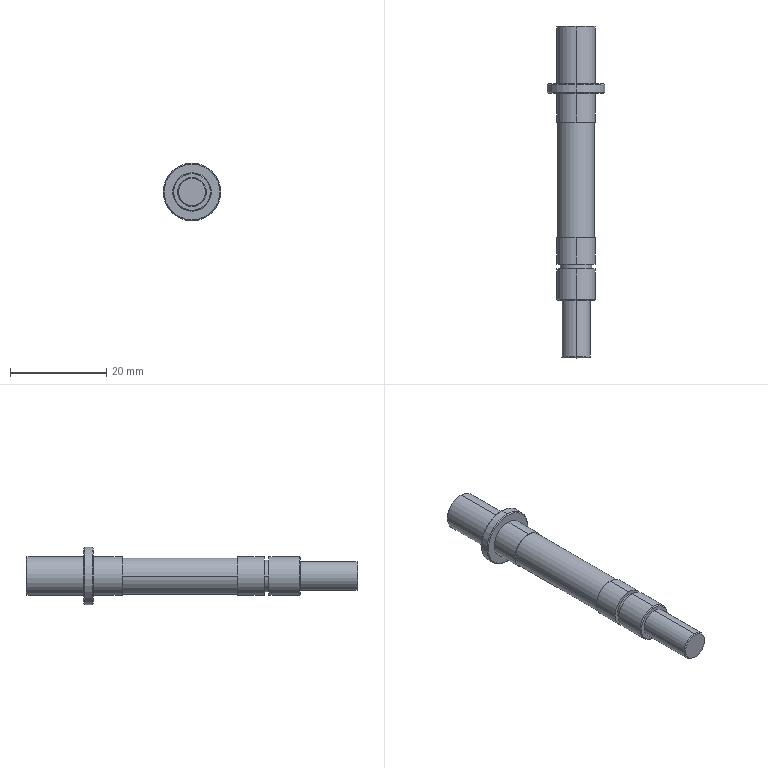Part | SolidWorks | features ICE 3, Chamfer 1, Extrusion 1, RevCut 1 | 1 solid | 35 faces | box 12 x 69 x 12 mm | volume 3193 mm3 | cylinder 16 | cone 10 | plane 9 | commonest cylinder face diameters 8 x8 6 x2 6.5 x2 7.6 x2 12 x2
STEP:
#1=CARTESIAN_POINT('',(0.,43.,-5.8));
#2=VERTEX_POINT('',#1);
#3=CARTESIAN_POINT('',(0.,43.,5.8));
#4=VERTEX_POINT('',#3);
#5=CARTESIAN_POINT('',(0.,43.,0.));
#6=DIRECTION('',(0.,-1.,0.));
#7=DIRECTION('',(0.,0.,1.));
#8=AXIS2_PLACEMENT_3D('',#5,#6,#7);
#9=CIRCLE('',#8,5.8);
#10=EDGE_CURVE('',#2,#4,#9,.T.);
#11=ORIENTED_EDGE('',*,*,#10,.F.);
#12=CARTESIAN_POINT('',(0.,43.2,-6.));
#13=VERTEX_POINT('',#12);
#14=CARTESIAN_POINT('',(0.,43.2,-6.));
#15=DIRECTION('',(0.,0.7071,-0.7071));
#16=VECTOR('',#15,1000.);
#17=LINE('',#14,#16);
#18=EDGE_CURVE('',#2,#13,#17,.T.);
#19=ORIENTED_EDGE('',*,*,#18,.T.);
#20=CARTESIAN_POINT('',(0.,43.2,6.));
#21=VERTEX_POINT('',#20);
#22=CARTESIAN_POINT('',(0.,43.2,0.));
#23=DIRECTION('',(0.,1.,0.));
#24=DIRECTION('',(0.,0.,1.));
#25=AXIS2_PLACEMENT_3D('',#22,#23,#24);
#26=CIRCLE('',#25,6.);
#27=EDGE_CURVE('',#21,#13,#26,.T.);
#28=ORIENTED_EDGE('',*,*,#27,.F.);
#29=CARTESIAN_POINT('',(0.,43.2,6.));
#30=DIRECTION('',(0.,0.7071,0.7071));
#31=VECTOR('',#30,1000.);
#32=LINE('',#29,#31);
#33=EDGE_CURVE('',#4,#21,#32,.T.);
#34=ORIENTED_EDGE('',*,*,#33,.F.);
#35=EDGE_LOOP('',(#11,#19,#28,#34));
#36=FACE_OUTER_BOUND('',#35,.T.);
#37=CARTESIAN_POINT('',(0.,43.2,0.));
#38=DIRECTION('',(0.,1.,0.));
#39=DIRECTION('',(0.,0.,1.));
#40=AXIS2_PLACEMENT_3D('',#37,#38,#39);
#41=CONICAL_SURFACE('',#40,6.,0.7854);
#42=ADVANCED_FACE('',(#36),#41,.T.);
#43=CARTESIAN_POINT('',(0.,0.,-3.8));
#44=VERTEX_POINT('',#43);
#45=CARTESIAN_POINT('',(0.,0.,3.8));
#46=VERTEX_POINT('',#45);
#47=CARTESIAN_POINT('',(0.,0.,0.));
#48=DIRECTION('',(0.,-1.,0.));
#49=DIRECTION('',(0.,0.,1.));
#50=AXIS2_PLACEMENT_3D('',#47,#48,#49);
#51=CIRCLE('',#50,3.8);
#52=EDGE_CURVE('',#44,#46,#51,.T.);
#53=ORIENTED_EDGE('',*,*,#52,.F.);
#54=CARTESIAN_POINT('',(0.,0.2,-4.));
#55=VERTEX_POINT('',#54);
#56=CARTESIAN_POINT('',(0.,0.2,-4.));
#57=DIRECTION('',(0.,0.7071,-0.7071));
#58=VECTOR('',#57,1000.);
#59=LINE('',#56,#58);
#60=EDGE_CURVE('',#44,#55,#59,.T.);
#61=ORIENTED_EDGE('',*,*,#60,.T.);
#62=CARTESIAN_POINT('',(0.,0.2,4.));
#63=VERTEX_POINT('',#62);
#64=CARTESIAN_POINT('',(0.,0.2,0.));
#65=DIRECTION('',(0.,1.,0.));
#66=DIRECTION('',(0.,0.,1.));
#67=AXIS2_PLACEMENT_3D('',#64,#65,#66);
#68=CIRCLE('',#67,4.);
#69=EDGE_CURVE('',#63,#55,#68,.T.);
#70=ORIENTED_EDGE('',*,*,#69,.F.);
#71=CARTESIAN_POINT('',(0.,0.2,4.));
#72=DIRECTION('',(0.,0.7071,0.7071));
#73=VECTOR('',#72,1000.);
#74=LINE('',#71,#73);
#75=EDGE_CURVE('',#46,#63,#74,.T.);
#76=ORIENTED_EDGE('',*,*,#75,.F.);
#77=EDGE_LOOP('',(#53,#61,#70,#76));
#78=FACE_OUTER_BOUND('',#77,.T.);
#79=CARTESIAN_POINT('',(0.,0.2,0.));
#80=DIRECTION('',(0.,1.,0.));
#81=DIRECTION('',(0.,0.,1.));
#82=AXIS2_PLACEMENT_3D('',#79,#80,#81);
#83=CONICAL_SURFACE('',#82,4.,0.7854);
#84=ADVANCED_FACE('',(#78),#83,.T.);
#85=CARTESIAN_POINT('',(0.,-12.,-2.8));
#86=VERTEX_POINT('',#85);
#87=CARTESIAN_POINT('',(0.,-12.,2.8));
#88=VERTEX_POINT('',#87);
#89=CARTESIAN_POINT('',(0.,-12.,0.));
#90=DIRECTION('',(0.,-1.,0.));
#91=DIRECTION('',(0.,0.,-1.));
#92=AXIS2_PLACEMENT_3D('',#89,#90,#91);
#93=CIRCLE('',#92,2.8);
#94=EDGE_CURVE('',#86,#88,#93,.T.);
#95=ORIENTED_EDGE('',*,*,#94,.F.);
#96=CARTESIAN_POINT('',(0.,-11.8,-3.));
#97=VERTEX_POINT('',#96);
#98=CARTESIAN_POINT('',(0.,-12.,-2.8));
#99=DIRECTION('',(0.,0.7071,-0.7071));
#100=VECTOR('',#99,1000.);
#101=LINE('',#98,#100);
#102=EDGE_CURVE('',#86,#97,#101,.T.);
#103=ORIENTED_EDGE('',*,*,#102,.T.);
#104=CARTESIAN_POINT('',(0.,-11.8,3.));
#105=VERTEX_POINT('',#104);
#106=CARTESIAN_POINT('',(0.,-11.8,0.));
#107=DIRECTION('',(0.,1.,0.));
#108=DIRECTION('',(0.,0.,-1.));
#109=AXIS2_PLACEMENT_3D('',#106,#107,#108);
#110=CIRCLE('',#109,3.);
#111=EDGE_CURVE('',#105,#97,#110,.T.);
#112=ORIENTED_EDGE('',*,*,#111,.F.);
#113=CARTESIAN_POINT('',(0.,-12.,2.8));
#114=DIRECTION('',(0.,0.7071,0.7071));
#115=VECTOR('',#114,1000.);
#116=LINE('',#113,#115);
#117=EDGE_CURVE('',#88,#105,#116,.T.);
#118=ORIENTED_EDGE('',*,*,#117,.F.);
#119=EDGE_LOOP('',(#95,#103,#112,#118));
#120=FACE_OUTER_BOUND('',#119,.T.);
#121=CARTESIAN_POINT('',(0.,-12.,0.));
#122=DIRECTION('',(0.,1.,0.));
#123=DIRECTION('',(0.,0.,1.));
#124=AXIS2_PLACEMENT_3D('',#121,#122,#123);
#125=CONICAL_SURFACE('',#124,2.8,0.7854);
#126=ADVANCED_FACE('',(#120),#125,.T.);
#127=CARTESIAN_POINT('',(0.,57.,3.8));
#128=VERTEX_POINT('',#127);
#129=CARTESIAN_POINT('',(0.,57.,-3.8));
#130=VERTEX_POINT('',#129);
#131=CARTESIAN_POINT('',(0.,57.,0.));
#132=DIRECTION('',(0.,1.,0.));
#133=DIRECTION('',(0.,0.,1.));
#134=AXIS2_PLACEMENT_3D('',#131,#132,#133);
#135=CIRCLE('',#134,3.8);
#136=EDGE_CURVE('',#128,#130,#135,.T.);
#137=ORIENTED_EDGE('',*,*,#136,.F.);
#138=CARTESIAN_POINT('',(0.,56.8,4.));
#139=VERTEX_POINT('',#138);
#140=CARTESIAN_POINT('',(0.,57.,3.8));
#141=DIRECTION('',(0.,-0.7071,0.7071));
#142=VECTOR('',#141,1000.);
#143=LINE('',#140,#142);
#144=EDGE_CURVE('',#128,#139,#143,.T.);
#145=ORIENTED_EDGE('',*,*,#144,.T.);
#146=CARTESIAN_POINT('',(0.,56.8,-4.));
#147=VERTEX_POINT('',#146);
#148=CARTESIAN_POINT('',(0.,56.8,0.));
#149=DIRECTION('',(0.,-1.,0.));
#150=DIRECTION('',(0.,0.,1.));
#151=AXIS2_PLACEMENT_3D('',#148,#149,#150);
#152=CIRCLE('',#151,4.);
#153=EDGE_CURVE('',#147,#139,#152,.T.);
#154=ORIENTED_EDGE('',*,*,#153,.F.);
#155=CARTESIAN_POINT('',(0.,57.,-3.8));
#156=DIRECTION('',(0.,-0.7071,-0.7071));
#157=VECTOR('',#156,1000.);
#158=LINE('',#155,#157);
#159=EDGE_CURVE('',#130,#147,#158,.T.);
#160=ORIENTED_EDGE('',*,*,#159,.F.);
#161=EDGE_LOOP('',(#137,#145,#154,#160));
#162=FACE_OUTER_BOUND('',#161,.T.);
#163=CARTESIAN_POINT('',(0.,57.,0.));
#164=DIRECTION('',(0.,-1.,0.));
#165=DIRECTION('',(0.,0.,-1.));
#166=AXIS2_PLACEMENT_3D('',#163,#164,#165);
#167=CONICAL_SURFACE('',#166,3.8,0.7854);
#168=ADVANCED_FACE('',(#162),#167,.T.);
#169=CARTESIAN_POINT('',(0.,45.,5.8));
#170=VERTEX_POINT('',#169);
#171=CARTESIAN_POINT('',(0.,45.,-5.8));
#172=VERTEX_POINT('',#171);
#173=CARTESIAN_POINT('',(0.,45.,0.));
#174=DIRECTION('',(0.,1.,0.));
#175=DIRECTION('',(0.,0.,1.));
#176=AXIS2_PLACEMENT_3D('',#173,#174,#175);
#177=CIRCLE('',#176,5.8);
#178=EDGE_CURVE('',#170,#172,#177,.T.);
#179=ORIENTED_EDGE('',*,*,#178,.F.);
#180=CARTESIAN_POINT('',(0.,44.8,6.));
#181=VERTEX_POINT('',#180);
#182=CARTESIAN_POINT('',(0.,45.,5.8));
#183=DIRECTION('',(0.,-0.7071,0.7071));
#184=VECTOR('',#183,1000.);
#185=LINE('',#182,#184);
#186=EDGE_CURVE('',#170,#181,#185,.T.);
#187=ORIENTED_EDGE('',*,*,#186,.T.);
#188=CARTESIAN_POINT('',(0.,44.8,-6.));
#189=VERTEX_POINT('',#188);
#190=CARTESIAN_POINT('',(0.,44.8,0.));
#191=DIRECTION('',(0.,-1.,0.));
#192=DIRECTION('',(0.,0.,1.));
#193=AXIS2_PLACEMENT_3D('',#190,#191,#192);
#194=CIRCLE('',#193,6.);
#195=EDGE_CURVE('',#189,#181,#194,.T.);
#196=ORIENTED_EDGE('',*,*,#195,.F.);
#197=CARTESIAN_POINT('',(0.,45.,-5.8));
#198=DIRECTION('',(0.,-0.7071,-0.7071));
#199=VECTOR('',#198,1000.);
#200=LINE('',#197,#199);
#201=EDGE_CURVE('',#172,#189,#200,.T.);
#202=ORIENTED_EDGE('',*,*,#201,.F.);
#203=EDGE_LOOP('',(#179,#187,#196,#202));
#204=FACE_OUTER_BOUND('',#203,.T.);
#205=CARTESIAN_POINT('',(0.,45.,0.));
#206=DIRECTION('',(0.,-1.,0.));
#207=DIRECTION('',(0.,0.,-1.));
#208=AXIS2_PLACEMENT_3D('',#205,#206,#207);
#209=CONICAL_SURFACE('',#208,5.8,0.7854);
#210=ADVANCED_FACE('',(#204),#209,.T.);
#211=ORIENTED_EDGE('',*,*,#111,.T.);
#212=CARTESIAN_POINT('',(0.,0.,-3.));
#213=VERTEX_POINT('',#212);
#214=CARTESIAN_POINT('',(0.,-12.,-3.));
#215=DIRECTION('',(0.,1.,0.));
#216=VECTOR('',#215,1000.);
#217=LINE('',#214,#216);
#218=EDGE_CURVE('',#97,#213,#217,.T.);
#219=ORIENTED_EDGE('',*,*,#218,.T.);
#220=CARTESIAN_POINT('',(0.,0.,3.));
#221=VERTEX_POINT('',#220);
#222=CARTESIAN_POINT('',(0.,0.,0.));
#223=DIRECTION('',(0.,-1.,0.));
#224=DIRECTION('',(0.,0.,1.));
#225=AXIS2_PLACEMENT_3D('',#222,#223,#224);
#226=CIRCLE('',#225,3.);
#227=EDGE_CURVE('',#213,#221,#226,.T.);
#228=ORIENTED_EDGE('',*,*,#227,.T.);
#229=CARTESIAN_POINT('',(0.,-12.,3.));
#230=DIRECTION('',(0.,1.,0.));
#231=VECTOR('',#230,1000.);
#232=LINE('',#229,#231);
#233=EDGE_CURVE('',#105,#221,#232,.T.);
#234=ORIENTED_EDGE('',*,*,#233,.F.);
#235=EDGE_LOOP('',(#211,#219,#228,#234));
#236=FACE_OUTER_BOUND('',#235,.T.);
#237=CARTESIAN_POINT('',(0.,-12.,0.));
#238=DIRECTION('',(0.,1.,0.));
#239=DIRECTION('',(0.,0.,1.));
#240=AXIS2_PLACEMENT_3D('',#237,#238,#239);
#241=CYLINDRICAL_SURFACE('',#240,3.);
#242=ADVANCED_FACE('',(#236),#241,.T.);
#243=CARTESIAN_POINT('',(0.,6.5,-4.));
#244=VERTEX_POINT('',#243);
#245=CARTESIAN_POINT('',(0.,6.5,4.));
#246=VERTEX_POINT('',#245);
#247=CARTESIAN_POINT('',(0.,6.5,0.));
#248=DIRECTION('',(0.,-1.,0.));
#249=DIRECTION('',(1.,0.,0.));
#250=AXIS2_PLACEMENT_3D('',#247,#248,#249);
#251=CIRCLE('',#250,4.);
#252=EDGE_CURVE('',#244,#246,#251,.T.);
#253=ORIENTED_EDGE('',*,*,#252,.T.);
#254=CARTESIAN_POINT('',(0.,43.,4.));
#255=DIRECTION('',(0.,-1.,0.));
#256=VECTOR('',#255,1000.);
#257=LINE('',#254,#256);
#258=EDGE_CURVE('',#246,#63,#257,.T.);
#259=ORIENTED_EDGE('',*,*,#258,.T.);
#260=ORIENTED_EDGE('',*,*,#69,.T.);
#261=CARTESIAN_POINT('',(0.,43.,-4.));
#262=DIRECTION('',(0.,-1.,0.));
#263=VECTOR('',#262,1000.);
#264=LINE('',#261,#263);
#265=EDGE_CURVE('',#244,#55,#264,.T.);
#266=ORIENTED_EDGE('',*,*,#265,.F.);
#267=EDGE_LOOP('',(#253,#259,#260,#266));
#268=FACE_OUTER_BOUND('',#267,.T.);
#269=CARTESIAN_POINT('',(0.,43.,0.));
#270=DIRECTION('',(0.,-1.,0.));
#271=DIRECTION('',(0.,0.,-1.));
#272=AXIS2_PLACEMENT_3D('',#269,#270,#271);
#273=CYLINDRICAL_SURFACE('',#272,4.);
#274=ADVANCED_FACE('',(#268),#273,.T.);
#275=CARTESIAN_POINT('',(3.25,7.5,0.));
#276=VERTEX_POINT('',#275);
#277=CARTESIAN_POINT('',(-3.25,7.5,0.));
#278=VERTEX_POINT('',#277);
#279=CARTESIAN_POINT('',(0.,7.5,0.));
#280=DIRECTION('',(0.,-1.,0.));
#281=DIRECTION('',(1.,0.,0.));
#282=AXIS2_PLACEMENT_3D('',#279,#280,#281);
#283=CIRCLE('',#282,3.25);
#284=EDGE_CURVE('',#276,#278,#283,.T.);
#285=ORIENTED_EDGE('',*,*,#284,.T.);
#286=CARTESIAN_POINT('',(-3.25,6.5,0.));
#287=VERTEX_POINT('',#286);
#288=CARTESIAN_POINT('',(-3.25,0.,0.));
#289=DIRECTION('',(0.,-1.,0.));
#290=VECTOR('',#289,1000.);
#291=LINE('',#288,#290);
#292=EDGE_CURVE('',#278,#287,#291,.T.);
#293=ORIENTED_EDGE('',*,*,#292,.T.);
#294=CARTESIAN_POINT('',(3.25,6.5,0.));
#295=VERTEX_POINT('',#294);
#296=CARTESIAN_POINT('',(0.,6.5,0.));
#297=DIRECTION('',(0.,-1.,0.));
#298=DIRECTION('',(1.,0.,0.));
#299=AXIS2_PLACEMENT_3D('',#296,#297,#298);
#300=CIRCLE('',#299,3.25);
#301=EDGE_CURVE('',#295,#287,#300,.T.);
#302=ORIENTED_EDGE('',*,*,#301,.F.);
#303=CARTESIAN_POINT('',(3.25,0.,0.));
#304=DIRECTION('',(0.,-1.,0.));
#305=VECTOR('',#304,1000.);
#306=LINE('',#303,#305);
#307=EDGE_CURVE('',#276,#295,#306,.T.);
#308=ORIENTED_EDGE('',*,*,#307,.F.);
#309=EDGE_LOOP('',(#285,#293,#302,#308));
#310=FACE_OUTER_BOUND('',#309,.T.);
#311=CARTESIAN_POINT('',(0.,0.,0.));
#312=DIRECTION('',(0.,-1.,0.));
#313=DIRECTION('',(1.,0.,0.));
#314=AXIS2_PLACEMENT_3D('',#311,#312,#313);
#315=CYLINDRICAL_SURFACE('',#314,3.25);
#316=ADVANCED_FACE('',(#310),#315,.T.);
#317=CARTESIAN_POINT('',(0.,13.,-4.));
#318=VERTEX_POINT('',#317);
#319=CARTESIAN_POINT('',(0.,13.,4.));
#320=VERTEX_POINT('',#319);
#321=CARTESIAN_POINT('',(0.,13.,0.));
#322=DIRECTION('',(0.,-1.,0.));
#323=DIRECTION('',(1.,0.,0.));
#324=AXIS2_PLACEMENT_3D('',#321,#322,#323);
#325=CIRCLE('',#324,4.);
#326=EDGE_CURVE('',#318,#320,#325,.T.);
#327=ORIENTED_EDGE('',*,*,#326,.T.);
#328=CARTESIAN_POINT('',(0.,7.5,4.));
#329=VERTEX_POINT('',#328);
#330=CARTESIAN_POINT('',(0.,43.,4.));
#331=DIRECTION('',(0.,-1.,0.));
#332=VECTOR('',#331,1000.);
#333=LINE('',#330,#332);
#334=EDGE_CURVE('',#320,#329,#333,.T.);
#335=ORIENTED_EDGE('',*,*,#334,.T.);
#336=CARTESIAN_POINT('',(0.,7.5,-4.));
#337=VERTEX_POINT('',#336);
#338=CARTESIAN_POINT('',(0.,7.5,0.));
#339=DIRECTION('',(0.,1.,0.));
#340=DIRECTION('',(-1.,0.,0.));
#341=AXIS2_PLACEMENT_3D('',#338,#339,#340);
#342=CIRCLE('',#341,4.);
#343=EDGE_CURVE('',#329,#337,#342,.T.);
#344=ORIENTED_EDGE('',*,*,#343,.T.);
#345=CARTESIAN_POINT('',(0.,43.,-4.));
#346=DIRECTION('',(0.,-1.,0.));
#347=VECTOR('',#346,1000.);
#348=LINE('',#345,#347);
#349=EDGE_CURVE('',#318,#337,#348,.T.);
#350=ORIENTED_EDGE('',*,*,#349,.F.);
#351=EDGE_LOOP('',(#327,#335,#344,#350));
#352=FACE_OUTER_BOUND('',#351,.T.);
#353=CARTESIAN_POINT('',(0.,43.,0.));
#354=DIRECTION('',(0.,-1.,0.));
#355=DIRECTION('',(0.,0.,-1.));
#356=AXIS2_PLACEMENT_3D('',#353,#354,#355);
#357=CYLINDRICAL_SURFACE('',#356,4.);
#358=ADVANCED_FACE('',(#352),#357,.T.);
#359=CARTESIAN_POINT('',(3.8,37.,0.));
#360=VERTEX_POINT('',#359);
#361=CARTESIAN_POINT('',(-3.8,37.,0.));
#362=VERTEX_POINT('',#361);
#363=CARTESIAN_POINT('',(0.,37.,0.));
#364=DIRECTION('',(0.,-1.,0.));
#365=DIRECTION('',(1.,0.,0.));
#366=AXIS2_PLACEMENT_3D('',#363,#364,#365);
#367=CIRCLE('',#366,3.8);
#368=EDGE_CURVE('',#360,#362,#367,.T.);
#369=ORIENTED_EDGE('',*,*,#368,.T.);
#370=CARTESIAN_POINT('',(-3.8,13.,0.));
#371=VERTEX_POINT('',#370);
#372=CARTESIAN_POINT('',(-3.8,0.,0.));
#373=DIRECTION('',(0.,-1.,0.));
#374=VECTOR('',#373,1000.);
#375=LINE('',#372,#374);
#376=EDGE_CURVE('',#362,#371,#375,.T.);
#377=ORIENTED_EDGE('',*,*,#376,.T.);
#378=CARTESIAN_POINT('',(3.8,13.,0.));
#379=VERTEX_POINT('',#378);
#380=CARTESIAN_POINT('',(0.,13.,0.));
#381=DIRECTION('',(0.,-1.,0.));
#382=DIRECTION('',(1.,0.,0.));
#383=AXIS2_PLACEMENT_3D('',#380,#381,#382);
#384=CIRCLE('',#383,3.8);
#385=EDGE_CURVE('',#379,#371,#384,.T.);
#386=ORIENTED_EDGE('',*,*,#385,.F.);
#387=CARTESIAN_POINT('',(3.8,0.,0.));
#388=DIRECTION('',(0.,-1.,0.));
#389=VECTOR('',#388,1000.);
#390=LINE('',#387,#389);
#391=EDGE_CURVE('',#360,#379,#390,.T.);
#392=ORIENTED_EDGE('',*,*,#391,.F.);
#393=EDGE_LOOP('',(#369,#377,#386,#392));
#394=FACE_OUTER_BOUND('',#393,.T.);
#395=CARTESIAN_POINT('',(0.,0.,0.));
#396=DIRECTION('',(0.,-1.,0.));
#397=DIRECTION('',(1.,0.,0.));
#398=AXIS2_PLACEMENT_3D('',#395,#396,#397);
#399=CYLINDRICAL_SURFACE('',#398,3.8);
#400=ADVANCED_FACE('',(#394),#399,.T.);
#401=ORIENTED_EDGE('',*,*,#153,.T.);
#402=CARTESIAN_POINT('',(0.,45.,4.));
#403=VERTEX_POINT('',#402);
#404=CARTESIAN_POINT('',(0.,57.,4.));
#405=DIRECTION('',(0.,-1.,0.));
#406=VECTOR('',#405,1000.);
#407=LINE('',#404,#406);
#408=EDGE_CURVE('',#139,#403,#407,.T.);
#409=ORIENTED_EDGE('',*,*,#408,.T.);
#410=CARTESIAN_POINT('',(0.,45.,-4.));
#411=VERTEX_POINT('',#410);
#412=CARTESIAN_POINT('',(0.,45.,0.));
#413=DIRECTION('',(0.,1.,0.));
#414=DIRECTION('',(0.,0.,1.));
#415=AXIS2_PLACEMENT_3D('',#412,#413,#414);
#416=CIRCLE('',#415,4.);
#417=EDGE_CURVE('',#403,#411,#416,.T.);
#418=ORIENTED_EDGE('',*,*,#417,.T.);
#419=CARTESIAN_POINT('',(0.,57.,-4.));
#420=DIRECTION('',(0.,-1.,0.));
#421=VECTOR('',#420,1000.);
#422=LINE('',#419,#421);
#423=EDGE_CURVE('',#147,#411,#422,.T.);
#424=ORIENTED_EDGE('',*,*,#423,.F.);
#425=EDGE_LOOP('',(#401,#409,#418,#424));
#426=FACE_OUTER_BOUND('',#425,.T.);
#427=CARTESIAN_POINT('',(0.,57.,0.));
#428=DIRECTION('',(0.,-1.,0.));
#429=DIRECTION('',(0.,0.,-1.));
#430=AXIS2_PLACEMENT_3D('',#427,#428,#429);
#431=CYLINDRICAL_SURFACE('',#430,4.);
#432=ADVANCED_FACE('',(#426),#431,.T.);
#433=ORIENTED_EDGE('',*,*,#195,.T.);
#434=CARTESIAN_POINT('',(0.,45.,6.));
#435=DIRECTION('',(0.,-1.,0.));
#436=VECTOR('',#435,1000.);
#437=LINE('',#434,#436);
#438=EDGE_CURVE('',#181,#21,#437,.T.);
#439=ORIENTED_EDGE('',*,*,#438,.T.);
#440=ORIENTED_EDGE('',*,*,#27,.T.);
#441=CARTESIAN_POINT('',(0.,45.,-6.));
#442=DIRECTION('',(0.,-1.,0.));
#443=VECTOR('',#442,1000.);
#444=LINE('',#441,#443);
#445=EDGE_CURVE('',#189,#13,#444,.T.);
#446=ORIENTED_EDGE('',*,*,#445,.F.);
#447=EDGE_LOOP('',(#433,#439,#440,#446));
#448=FACE_OUTER_BOUND('',#447,.T.);
#449=CARTESIAN_POINT('',(0.,45.,0.));
#450=DIRECTION('',(0.,-1.,0.));
#451=DIRECTION('',(0.,0.,-1.));
#452=AXIS2_PLACEMENT_3D('',#449,#450,#451);
#453=CYLINDRICAL_SURFACE('',#452,6.);
#454=ADVANCED_FACE('',(#448),#453,.T.);
#455=CARTESIAN_POINT('',(0.,43.,4.));
#456=VERTEX_POINT('',#455);
#457=CARTESIAN_POINT('',(0.,43.,-4.));
#458=VERTEX_POINT('',#457);
#459=CARTESIAN_POINT('',(0.,43.,0.));
#460=DIRECTION('',(0.,1.,0.));
#461=DIRECTION('',(0.,0.,1.));
#462=AXIS2_PLACEMENT_3D('',#459,#460,#461);
#463=CIRCLE('',#462,4.);
#464=EDGE_CURVE('',#456,#458,#463,.T.);
#465=ORIENTED_EDGE('',*,*,#464,.F.);
#466=CARTESIAN_POINT('',(0.,37.,4.));
#467=VERTEX_POINT('',#466);
#468=CARTESIAN_POINT('',(0.,43.,4.));
#469=DIRECTION('',(0.,-1.,0.));
#470=VECTOR('',#469,1000.);
#471=LINE('',#468,#470);
#472=EDGE_CURVE('',#456,#467,#471,.T.);
#473=ORIENTED_EDGE('',*,*,#472,.T.);
#474=CARTESIAN_POINT('',(0.,37.,-4.));
#475=VERTEX_POINT('',#474);
#476=CARTESIAN_POINT('',(0.,37.,0.));
#477=DIRECTION('',(0.,1.,0.));
#478=DIRECTION('',(-1.,0.,0.));
#479=AXIS2_PLACEMENT_3D('',#476,#477,#478);
#480=CIRCLE('',#479,4.);
#481=EDGE_CURVE('',#467,#475,#480,.T.);
#482=ORIENTED_EDGE('',*,*,#481,.T.);
#483=CARTESIAN_POINT('',(0.,43.,-4.));
#484=DIRECTION('',(0.,-1.,0.));
#485=VECTOR('',#484,1000.);
#486=LINE('',#483,#485);
#487=EDGE_CURVE('',#458,#475,#486,.T.);
#488=ORIENTED_EDGE('',*,*,#487,.F.);
#489=EDGE_LOOP('',(#465,#473,#482,#488));
#490=FACE_OUTER_BOUND('',#489,.T.);
#491=CARTESIAN_POINT('',(0.,43.,0.));
#492=DIRECTION('',(0.,-1.,0.));
#493=DIRECTION('',(0.,0.,-1.));
#494=AXIS2_PLACEMENT_3D('',#491,#492,#493);
#495=CYLINDRICAL_SURFACE('',#494,4.);
#496=ADVANCED_FACE('',(#490),#495,.T.);
#497=CARTESIAN_POINT('',(0.,0.,0.));
#498=DIRECTION('',(0.,-1.,0.));
#499=DIRECTION('',(0.,0.,1.));
#500=AXIS2_PLACEMENT_3D('',#497,#498,#499);
#501=CIRCLE('',#500,3.8);
#502=EDGE_CURVE('',#46,#44,#501,.T.);
#503=ORIENTED_EDGE('',*,*,#502,.T.);
#504=ORIENTED_EDGE('',*,*,#52,.T.);
#505=EDGE_LOOP('',(#503,#504));
#506=FACE_OUTER_BOUND('',#505,.T.);
#507=CARTESIAN_POINT('',(0.,0.,0.));
#508=DIRECTION('',(0.,-1.,0.));
#509=DIRECTION('',(0.,0.,1.));
#510=AXIS2_PLACEMENT_3D('',#507,#508,#509);
#511=CIRCLE('',#510,3.);
#512=EDGE_CURVE('',#221,#213,#511,.T.);
#513=ORIENTED_EDGE('',*,*,#512,.F.);
#514=ORIENTED_EDGE('',*,*,#227,.F.);
#515=EDGE_LOOP('',(#513,#514));
#516=FACE_BOUND('',#515,.T.);
#517=CARTESIAN_POINT('',(0.,0.,0.));
#518=DIRECTION('',(0.,1.,0.));
#519=DIRECTION('',(0.,0.,1.));
#520=AXIS2_PLACEMENT_3D('',#517,#518,#519);
#521=PLANE('',#520);
#522=ADVANCED_FACE('',(#506,#516),#521,.F.);
#523=CARTESIAN_POINT('',(0.,45.,0.));
#524=DIRECTION('',(0.,1.,0.));
#525=DIRECTION('',(0.,0.,1.));
#526=AXIS2_PLACEMENT_3D('',#523,#524,#525);
#527=CIRCLE('',#526,5.8);
#528=EDGE_CURVE('',#172,#170,#527,.T.);
#529=ORIENTED_EDGE('',*,*,#528,.T.);
#530=ORIENTED_EDGE('',*,*,#178,.T.);
#531=EDGE_LOOP('',(#529,#530));
#532=FACE_OUTER_BOUND('',#531,.T.);
#533=CARTESIAN_POINT('',(0.,45.,0.));
#534=DIRECTION('',(0.,1.,0.));
#535=DIRECTION('',(0.,0.,1.));
#536=AXIS2_PLACEMENT_3D('',#533,#534,#535);
#537=CIRCLE('',#536,4.);
#538=EDGE_CURVE('',#411,#403,#537,.T.);
#539=ORIENTED_EDGE('',*,*,#538,.F.);
#540=ORIENTED_EDGE('',*,*,#417,.F.);
#541=EDGE_LOOP('',(#539,#540));
#542=FACE_BOUND('',#541,.T.);
#543=CARTESIAN_POINT('',(0.,45.,0.));
#544=DIRECTION('',(0.,1.,0.));
#545=DIRECTION('',(0.,0.,1.));
#546=AXIS2_PLACEMENT_3D('',#543,#544,#545);
#547=PLANE('',#546);
#548=ADVANCED_FACE('',(#532,#542),#547,.T.);
#549=ORIENTED_EDGE('',*,*,#472,.F.);
#550=CARTESIAN_POINT('',(0.,43.,0.));
#551=DIRECTION('',(0.,1.,0.));
#552=DIRECTION('',(0.,0.,1.));
#553=AXIS2_PLACEMENT_3D('',#550,#551,#552);
#554=CIRCLE('',#553,4.);
#555=EDGE_CURVE('',#458,#456,#554,.T.);
#556=ORIENTED_EDGE('',*,*,#555,.F.);
#557=ORIENTED_EDGE('',*,*,#487,.T.);
#558=CARTESIAN_POINT('',(0.,37.,0.));
#559=DIRECTION('',(0.,1.,0.));
#560=DIRECTION('',(-1.,0.,0.));
#561=AXIS2_PLACEMENT_3D('',#558,#559,#560);
#562=CIRCLE('',#561,4.);
#563=EDGE_CURVE('',#475,#467,#562,.T.);
#564=ORIENTED_EDGE('',*,*,#563,.T.);
#565=EDGE_LOOP('',(#549,#556,#557,#564));
#566=FACE_OUTER_BOUND('',#565,.T.);
#567=CARTESIAN_POINT('',(0.,43.,0.));
#568=DIRECTION('',(0.,-1.,0.));
#569=DIRECTION('',(0.,0.,-1.));
#570=AXIS2_PLACEMENT_3D('',#567,#568,#569);
#571=CYLINDRICAL_SURFACE('',#570,4.);
#572=ADVANCED_FACE('',(#566),#571,.T.);
#573=CARTESIAN_POINT('',(0.,43.,0.));
#574=DIRECTION('',(0.,-1.,0.));
#575=DIRECTION('',(0.,0.,1.));
#576=AXIS2_PLACEMENT_3D('',#573,#574,#575);
#577=CIRCLE('',#576,5.8);
#578=EDGE_CURVE('',#4,#2,#577,.T.);
#579=ORIENTED_EDGE('',*,*,#578,.T.);
#580=ORIENTED_EDGE('',*,*,#10,.T.);
#581=EDGE_LOOP('',(#579,#580));
#582=FACE_OUTER_BOUND('',#581,.T.);
#583=ORIENTED_EDGE('',*,*,#555,.T.);
#584=ORIENTED_EDGE('',*,*,#464,.T.);
#585=EDGE_LOOP('',(#583,#584));
#586=FACE_BOUND('',#585,.T.);
#587=CARTESIAN_POINT('',(0.,43.,0.));
#588=DIRECTION('',(0.,1.,0.));
#589=DIRECTION('',(0.,0.,1.));
#590=AXIS2_PLACEMENT_3D('',#587,#588,#589);
#591=PLANE('',#590);
#592=ADVANCED_FACE('',(#582,#586),#591,.F.);
#593=ORIENTED_EDGE('',*,*,#438,.F.);
#594=CARTESIAN_POINT('',(0.,44.8,0.));
#595=DIRECTION('',(0.,-1.,0.));
#596=DIRECTION('',(0.,0.,1.));
#597=AXIS2_PLACEMENT_3D('',#594,#595,#596);
#598=CIRCLE('',#597,6.);
#599=EDGE_CURVE('',#181,#189,#598,.T.);
#600=ORIENTED_EDGE('',*,*,#599,.T.);
#601=ORIENTED_EDGE('',*,*,#445,.T.);
#602=CARTESIAN_POINT('',(0.,43.2,0.));
#603=DIRECTION('',(0.,1.,0.));
#604=DIRECTION('',(0.,0.,1.));
#605=AXIS2_PLACEMENT_3D('',#602,#603,#604);
#606=CIRCLE('',#605,6.);
#607=EDGE_CURVE('',#13,#21,#606,.T.);
#608=ORIENTED_EDGE('',*,*,#607,.T.);
#609=EDGE_LOOP('',(#593,#600,#601,#608));
#610=FACE_OUTER_BOUND('',#609,.T.);
#611=CARTESIAN_POINT('',(0.,45.,0.));
#612=DIRECTION('',(0.,-1.,0.));
#613=DIRECTION('',(0.,0.,-1.));
#614=AXIS2_PLACEMENT_3D('',#611,#612,#613);
#615=CYLINDRICAL_SURFACE('',#614,6.);
#616=ADVANCED_FACE('',(#610),#615,.T.);
#617=ORIENTED_EDGE('',*,*,#408,.F.);
#618=CARTESIAN_POINT('',(0.,56.8,0.));
#619=DIRECTION('',(0.,-1.,0.));
#620=DIRECTION('',(0.,0.,1.));
#621=AXIS2_PLACEMENT_3D('',#618,#619,#620);
#622=CIRCLE('',#621,4.);
#623=EDGE_CURVE('',#139,#147,#622,.T.);
#624=ORIENTED_EDGE('',*,*,#623,.T.);
#625=ORIENTED_EDGE('',*,*,#423,.T.);
#626=ORIENTED_EDGE('',*,*,#538,.T.);
#627=EDGE_LOOP('',(#617,#624,#625,#626));
#628=FACE_OUTER_BOUND('',#627,.T.);
#629=CARTESIAN_POINT('',(0.,57.,0.));
#630=DIRECTION('',(0.,-1.,0.));
#631=DIRECTION('',(0.,0.,-1.));
#632=AXIS2_PLACEMENT_3D('',#629,#630,#631);
#633=CYLINDRICAL_SURFACE('',#632,4.);
#634=ADVANCED_FACE('',(#628),#633,.T.);
#635=CARTESIAN_POINT('',(0.,57.,0.));
#636=DIRECTION('',(0.,1.,0.));
#637=DIRECTION('',(0.,0.,1.));
#638=AXIS2_PLACEMENT_3D('',#635,#636,#637);
#639=CIRCLE('',#638,3.8);
#640=EDGE_CURVE('',#130,#128,#639,.T.);
#641=ORIENTED_EDGE('',*,*,#640,.T.);
#642=ORIENTED_EDGE('',*,*,#136,.T.);
#643=EDGE_LOOP('',(#641,#642));
#644=FACE_OUTER_BOUND('',#643,.T.);
#645=CARTESIAN_POINT('',(0.,57.,0.));
#646=DIRECTION('',(0.,1.,0.));
#647=DIRECTION('',(0.,0.,1.));
#648=AXIS2_PLACEMENT_3D('',#645,#646,#647);
#649=PLANE('',#648);
#650=ADVANCED_FACE('',(#644),#649,.T.);
#651=ORIENTED_EDGE('',*,*,#385,.T.);
#652=CARTESIAN_POINT('',(0.,13.,0.));
#653=DIRECTION('',(0.,-1.,0.));
#654=DIRECTION('',(1.,0.,0.));
#655=AXIS2_PLACEMENT_3D('',#652,#653,#654);
#656=CIRCLE('',#655,3.8);
#657=EDGE_CURVE('',#371,#379,#656,.T.);
#658=ORIENTED_EDGE('',*,*,#657,.T.);
#659=EDGE_LOOP('',(#651,#658));
#660=FACE_BOUND('',#659,.T.);
#661=ORIENTED_EDGE('',*,*,#326,.F.);
#662=CARTESIAN_POINT('',(0.,13.,0.));
#663=DIRECTION('',(0.,-1.,0.));
#664=DIRECTION('',(1.,0.,0.));
#665=AXIS2_PLACEMENT_3D('',#662,#663,#664);
#666=CIRCLE('',#665,4.);
#667=EDGE_CURVE('',#320,#318,#666,.T.);
#668=ORIENTED_EDGE('',*,*,#667,.F.);
#669=EDGE_LOOP('',(#661,#668));
#670=FACE_OUTER_BOUND('',#669,.T.);
#671=CARTESIAN_POINT('',(3.8,13.,0.));
#672=DIRECTION('',(0.,-1.,0.));
#673=DIRECTION('',(1.,0.,0.));
#674=AXIS2_PLACEMENT_3D('',#671,#672,#673);
#675=PLANE('',#674);
#676=ADVANCED_FACE('',(#660,#670),#675,.F.);
#677=ORIENTED_EDGE('',*,*,#368,.F.);
#678=CARTESIAN_POINT('',(0.,37.,0.));
#679=DIRECTION('',(0.,-1.,0.));
#680=DIRECTION('',(1.,0.,0.));
#681=AXIS2_PLACEMENT_3D('',#678,#679,#680);
#682=CIRCLE('',#681,3.8);
#683=EDGE_CURVE('',#362,#360,#682,.T.);
#684=ORIENTED_EDGE('',*,*,#683,.F.);
#685=EDGE_LOOP('',(#677,#684));
#686=FACE_BOUND('',#685,.T.);
#687=ORIENTED_EDGE('',*,*,#563,.F.);
#688=ORIENTED_EDGE('',*,*,#481,.F.);
#689=EDGE_LOOP('',(#687,#688));
#690=FACE_OUTER_BOUND('',#689,.T.);
#691=CARTESIAN_POINT('',(3.8,37.,0.));
#692=DIRECTION('',(0.,1.,0.));
#693=DIRECTION('',(-1.,0.,0.));
#694=AXIS2_PLACEMENT_3D('',#691,#692,#693);
#695=PLANE('',#694);
#696=ADVANCED_FACE('',(#686,#690),#695,.F.);
#697=ORIENTED_EDGE('',*,*,#376,.F.);
#698=ORIENTED_EDGE('',*,*,#683,.T.);
#699=ORIENTED_EDGE('',*,*,#391,.T.);
#700=ORIENTED_EDGE('',*,*,#657,.F.);
#701=EDGE_LOOP('',(#697,#698,#699,#700));
#702=FACE_OUTER_BOUND('',#701,.T.);
#703=CARTESIAN_POINT('',(0.,0.,0.));
#704=DIRECTION('',(0.,-1.,0.));
#705=DIRECTION('',(1.,0.,0.));
#706=AXIS2_PLACEMENT_3D('',#703,#704,#705);
#707=CYLINDRICAL_SURFACE('',#706,3.8);
#708=ADVANCED_FACE('',(#702),#707,.T.);
#709=ORIENTED_EDGE('',*,*,#334,.F.);
#710=ORIENTED_EDGE('',*,*,#667,.T.);
#711=ORIENTED_EDGE('',*,*,#349,.T.);
#712=CARTESIAN_POINT('',(0.,7.5,0.));
#713=DIRECTION('',(0.,1.,0.));
#714=DIRECTION('',(-1.,0.,0.));
#715=AXIS2_PLACEMENT_3D('',#712,#713,#714);
#716=CIRCLE('',#715,4.);
#717=EDGE_CURVE('',#337,#329,#716,.T.);
#718=ORIENTED_EDGE('',*,*,#717,.T.);
#719=EDGE_LOOP('',(#709,#710,#711,#718));
#720=FACE_OUTER_BOUND('',#719,.T.);
#721=CARTESIAN_POINT('',(0.,43.,0.));
#722=DIRECTION('',(0.,-1.,0.));
#723=DIRECTION('',(0.,0.,-1.));
#724=AXIS2_PLACEMENT_3D('',#721,#722,#723);
#725=CYLINDRICAL_SURFACE('',#724,4.);
#726=ADVANCED_FACE('',(#720),#725,.T.);
#727=ORIENTED_EDGE('',*,*,#301,.T.);
#728=CARTESIAN_POINT('',(0.,6.5,0.));
#729=DIRECTION('',(0.,-1.,0.));
#730=DIRECTION('',(1.,0.,0.));
#731=AXIS2_PLACEMENT_3D('',#728,#729,#730);
#732=CIRCLE('',#731,3.25);
#733=EDGE_CURVE('',#287,#295,#732,.T.);
#734=ORIENTED_EDGE('',*,*,#733,.T.);
#735=EDGE_LOOP('',(#727,#734));
#736=FACE_BOUND('',#735,.T.);
#737=ORIENTED_EDGE('',*,*,#252,.F.);
#738=CARTESIAN_POINT('',(0.,6.5,0.));
#739=DIRECTION('',(0.,-1.,0.));
#740=DIRECTION('',(1.,0.,0.));
#741=AXIS2_PLACEMENT_3D('',#738,#739,#740);
#742=CIRCLE('',#741,4.);
#743=EDGE_CURVE('',#246,#244,#742,.T.);
#744=ORIENTED_EDGE('',*,*,#743,.F.);
#745=EDGE_LOOP('',(#737,#744));
#746=FACE_OUTER_BOUND('',#745,.T.);
#747=CARTESIAN_POINT('',(3.25,6.5,0.));
#748=DIRECTION('',(0.,-1.,0.));
#749=DIRECTION('',(1.,0.,0.));
#750=AXIS2_PLACEMENT_3D('',#747,#748,#749);
#751=PLANE('',#750);
#752=ADVANCED_FACE('',(#736,#746),#751,.F.);
#753=ORIENTED_EDGE('',*,*,#284,.F.);
#754=CARTESIAN_POINT('',(0.,7.5,0.));
#755=DIRECTION('',(0.,-1.,0.));
#756=DIRECTION('',(1.,0.,0.));
#757=AXIS2_PLACEMENT_3D('',#754,#755,#756);
#758=CIRCLE('',#757,3.25);
#759=EDGE_CURVE('',#278,#276,#758,.T.);
#760=ORIENTED_EDGE('',*,*,#759,.F.);
#761=EDGE_LOOP('',(#753,#760));
#762=FACE_BOUND('',#761,.T.);
#763=ORIENTED_EDGE('',*,*,#717,.F.);
#764=ORIENTED_EDGE('',*,*,#343,.F.);
#765=EDGE_LOOP('',(#763,#764));
#766=FACE_OUTER_BOUND('',#765,.T.);
#767=CARTESIAN_POINT('',(3.25,7.5,0.));
#768=DIRECTION('',(0.,1.,0.));
#769=DIRECTION('',(-1.,0.,0.));
#770=AXIS2_PLACEMENT_3D('',#767,#768,#769);
#771=PLANE('',#770);
#772=ADVANCED_FACE('',(#762,#766),#771,.F.);
#773=ORIENTED_EDGE('',*,*,#292,.F.);
#774=ORIENTED_EDGE('',*,*,#759,.T.);
#775=ORIENTED_EDGE('',*,*,#307,.T.);
#776=ORIENTED_EDGE('',*,*,#733,.F.);
#777=EDGE_LOOP('',(#773,#774,#775,#776));
#778=FACE_OUTER_BOUND('',#777,.T.);
#779=CARTESIAN_POINT('',(0.,0.,0.));
#780=DIRECTION('',(0.,-1.,0.));
#781=DIRECTION('',(1.,0.,0.));
#782=AXIS2_PLACEMENT_3D('',#779,#780,#781);
#783=CYLINDRICAL_SURFACE('',#782,3.25);
#784=ADVANCED_FACE('',(#778),#783,.T.);
#785=ORIENTED_EDGE('',*,*,#258,.F.);
#786=ORIENTED_EDGE('',*,*,#743,.T.);
#787=ORIENTED_EDGE('',*,*,#265,.T.);
#788=CARTESIAN_POINT('',(0.,0.2,0.));
#789=DIRECTION('',(0.,1.,0.));
#790=DIRECTION('',(0.,0.,1.));
#791=AXIS2_PLACEMENT_3D('',#788,#789,#790);
#792=CIRCLE('',#791,4.);
#793=EDGE_CURVE('',#55,#63,#792,.T.);
#794=ORIENTED_EDGE('',*,*,#793,.T.);
#795=EDGE_LOOP('',(#785,#786,#787,#794));
#796=FACE_OUTER_BOUND('',#795,.T.);
#797=CARTESIAN_POINT('',(0.,43.,0.));
#798=DIRECTION('',(0.,-1.,0.));
#799=DIRECTION('',(0.,0.,-1.));
#800=AXIS2_PLACEMENT_3D('',#797,#798,#799);
#801=CYLINDRICAL_SURFACE('',#800,4.);
#802=ADVANCED_FACE('',(#796),#801,.T.);
#803=ORIENTED_EDGE('',*,*,#218,.F.);
#804=CARTESIAN_POINT('',(0.,-11.8,0.));
#805=DIRECTION('',(0.,1.,0.));
#806=DIRECTION('',(0.,0.,-1.));
#807=AXIS2_PLACEMENT_3D('',#804,#805,#806);
#808=CIRCLE('',#807,3.);
#809=EDGE_CURVE('',#97,#105,#808,.T.);
#810=ORIENTED_EDGE('',*,*,#809,.T.);
#811=ORIENTED_EDGE('',*,*,#233,.T.);
#812=ORIENTED_EDGE('',*,*,#512,.T.);
#813=EDGE_LOOP('',(#803,#810,#811,#812));
#814=FACE_OUTER_BOUND('',#813,.T.);
#815=CARTESIAN_POINT('',(0.,-12.,0.));
#816=DIRECTION('',(0.,1.,0.));
#817=DIRECTION('',(0.,0.,1.));
#818=AXIS2_PLACEMENT_3D('',#815,#816,#817);
#819=CYLINDRICAL_SURFACE('',#818,3.);
#820=ADVANCED_FACE('',(#814),#819,.T.);
#821=CARTESIAN_POINT('',(0.,-12.,0.));
#822=DIRECTION('',(0.,-1.,0.));
#823=DIRECTION('',(0.,0.,-1.));
#824=AXIS2_PLACEMENT_3D('',#821,#822,#823);
#825=CIRCLE('',#824,2.8);
#826=EDGE_CURVE('',#88,#86,#825,.T.);
#827=ORIENTED_EDGE('',*,*,#826,.T.);
#828=ORIENTED_EDGE('',*,*,#94,.T.);
#829=EDGE_LOOP('',(#827,#828));
#830=FACE_OUTER_BOUND('',#829,.T.);
#831=CARTESIAN_POINT('',(0.,-12.,0.));
#832=DIRECTION('',(0.,-1.,0.));
#833=DIRECTION('',(0.,0.,-1.));
#834=AXIS2_PLACEMENT_3D('',#831,#832,#833);
#835=PLANE('',#834);
#836=ADVANCED_FACE('',(#830),#835,.T.);
#837=ORIENTED_EDGE('',*,*,#186,.F.);
#838=ORIENTED_EDGE('',*,*,#528,.F.);
#839=ORIENTED_EDGE('',*,*,#201,.T.);
#840=ORIENTED_EDGE('',*,*,#599,.F.);
#841=EDGE_LOOP('',(#837,#838,#839,#840));
#842=FACE_OUTER_BOUND('',#841,.T.);
#843=CARTESIAN_POINT('',(0.,45.,0.));
#844=DIRECTION('',(0.,-1.,0.));
#845=DIRECTION('',(0.,0.,-1.));
#846=AXIS2_PLACEMENT_3D('',#843,#844,#845);
#847=CONICAL_SURFACE('',#846,5.8,0.7854);
#848=ADVANCED_FACE('',(#842),#847,.T.);
#849=ORIENTED_EDGE('',*,*,#144,.F.);
#850=ORIENTED_EDGE('',*,*,#640,.F.);
#851=ORIENTED_EDGE('',*,*,#159,.T.);
#852=ORIENTED_EDGE('',*,*,#623,.F.);
#853=EDGE_LOOP('',(#849,#850,#851,#852));
#854=FACE_OUTER_BOUND('',#853,.T.);
#855=CARTESIAN_POINT('',(0.,57.,0.));
#856=DIRECTION('',(0.,-1.,0.));
#857=DIRECTION('',(0.,0.,-1.));
#858=AXIS2_PLACEMENT_3D('',#855,#856,#857);
#859=CONICAL_SURFACE('',#858,3.8,0.7854);
#860=ADVANCED_FACE('',(#854),#859,.T.);
#861=ORIENTED_EDGE('',*,*,#102,.F.);
#862=ORIENTED_EDGE('',*,*,#826,.F.);
#863=ORIENTED_EDGE('',*,*,#117,.T.);
#864=ORIENTED_EDGE('',*,*,#809,.F.);
#865=EDGE_LOOP('',(#861,#862,#863,#864));
#866=FACE_OUTER_BOUND('',#865,.T.);
#867=CARTESIAN_POINT('',(0.,-12.,0.));
#868=DIRECTION('',(0.,1.,0.));
#869=DIRECTION('',(0.,0.,1.));
#870=AXIS2_PLACEMENT_3D('',#867,#868,#869);
#871=CONICAL_SURFACE('',#870,2.8,0.7854);
#872=ADVANCED_FACE('',(#866),#871,.T.);
#873=ORIENTED_EDGE('',*,*,#60,.F.);
#874=ORIENTED_EDGE('',*,*,#502,.F.);
#875=ORIENTED_EDGE('',*,*,#75,.T.);
#876=ORIENTED_EDGE('',*,*,#793,.F.);
#877=EDGE_LOOP('',(#873,#874,#875,#876));
#878=FACE_OUTER_BOUND('',#877,.T.);
#879=CARTESIAN_POINT('',(0.,0.2,0.));
#880=DIRECTION('',(0.,1.,0.));
#881=DIRECTION('',(0.,0.,1.));
#882=AXIS2_PLACEMENT_3D('',#879,#880,#881);
#883=CONICAL_SURFACE('',#882,4.,0.7854);
#884=ADVANCED_FACE('',(#878),#883,.T.);
#885=ORIENTED_EDGE('',*,*,#18,.F.);
#886=ORIENTED_EDGE('',*,*,#578,.F.);
#887=ORIENTED_EDGE('',*,*,#33,.T.);
#888=ORIENTED_EDGE('',*,*,#607,.F.);
#889=EDGE_LOOP('',(#885,#886,#887,#888));
#890=FACE_OUTER_BOUND('',#889,.T.);
#891=CARTESIAN_POINT('',(0.,43.2,0.));
#892=DIRECTION('',(0.,1.,0.));
#893=DIRECTION('',(0.,0.,1.));
#894=AXIS2_PLACEMENT_3D('',#891,#892,#893);
#895=CONICAL_SURFACE('',#894,6.,0.7854);
#896=ADVANCED_FACE('',(#890),#895,.T.);
#897=CLOSED_SHELL('',(#42,#84,#126,#168,#210,#242,#274,#316,#358,#400,#432,#454,#496,#522,#548,#572,#592,#616,#634,#650,#676,#696,#708,#726,#752,#772,#784,#802,#820,#836,#848,#860,#872,#884,#896));
#898=MANIFOLD_SOLID_BREP('',#897);
#899=CARTESIAN_POINT('',(0.,0.,0.));
#900=DIRECTION('',(0.,0.,1.));
#901=DIRECTION('',(1.,0.,0.));
#902=AXIS2_PLACEMENT_3D('',#899,#900,#901);
#903=(LENGTH_UNIT()NAMED_UNIT(*)SI_UNIT(.MILLI.,.METRE.));
#904=UNCERTAINTY_MEASURE_WITH_UNIT(LENGTH_MEASURE(0.00001),#903,'','');
#905=(NAMED_UNIT(*)PLANE_ANGLE_UNIT()SI_UNIT($,.RADIAN.));
#906=(NAMED_UNIT(*)SI_UNIT($,.STERADIAN.)SOLID_ANGLE_UNIT());
#907=(GEOMETRIC_REPRESENTATION_CONTEXT(3)GLOBAL_UNCERTAINTY_ASSIGNED_CONTEXT((#904))GLOBAL_UNIT_ASSIGNED_CONTEXT((#903,#905,#906))REPRESENTATION_CONTEXT('',''));
#908=ADVANCED_BREP_SHAPE_REPRESENTATION('',(#898,#902),#907);